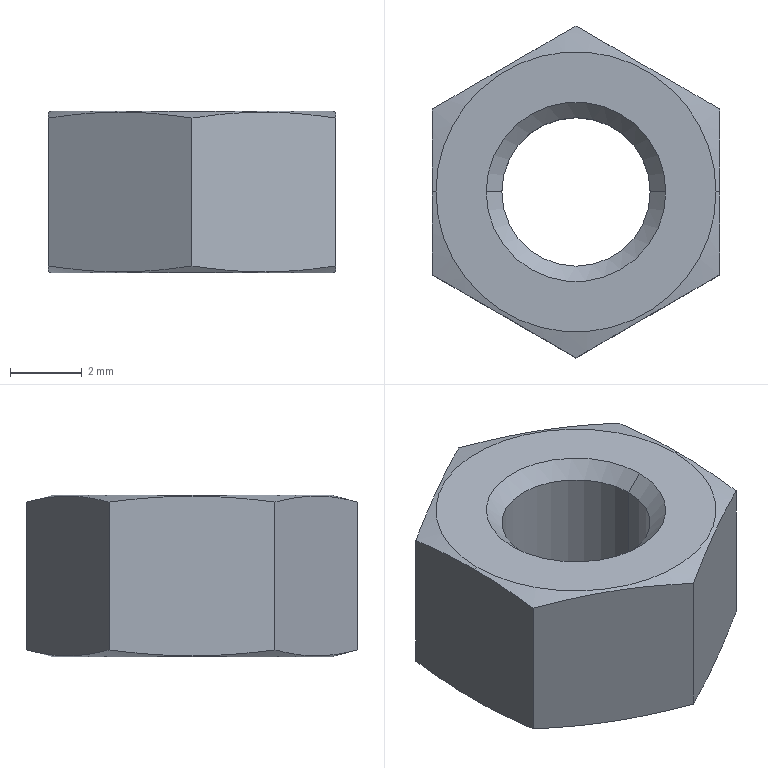Part | SolidWorks | features BaseBody 1 | 1 solid | 18 faces | box 8 x 9.238 x 4.5 mm | volume 185.536 mm3 | cone 8 | plane 8 | cylinder 2 | commonest cylinder face diameters 4.134 x2
STEP:
#1=CARTESIAN_POINT('',(-2.067,0.,-1.817));
#2=VERTEX_POINT('',#1);
#3=CARTESIAN_POINT('',(2.067,0.,-1.817));
#4=VERTEX_POINT('',#3);
#5=CARTESIAN_POINT('',(0.,0.,-1.817));
#6=DIRECTION('',(0.,0.,1.));
#7=DIRECTION('',(1.,0.,0.));
#8=AXIS2_PLACEMENT_3D('',#5,#6,#7);
#9=CIRCLE('',#8,2.067);
#10=EDGE_CURVE('',#2,#4,#9,.T.);
#11=ORIENTED_EDGE('',*,*,#10,.F.);
#12=CARTESIAN_POINT('',(-2.067,0.,1.817));
#13=VERTEX_POINT('',#12);
#14=CARTESIAN_POINT('',(-2.067,0.,-2.25));
#15=DIRECTION('',(0.,0.,1.));
#16=VECTOR('',#15,1000.);
#17=LINE('',#14,#16);
#18=EDGE_CURVE('',#2,#13,#17,.T.);
#19=ORIENTED_EDGE('',*,*,#18,.T.);
#20=CARTESIAN_POINT('',(2.067,0.,1.817));
#21=VERTEX_POINT('',#20);
#22=CARTESIAN_POINT('',(0.,0.,1.817));
#23=DIRECTION('',(0.,0.,-1.));
#24=DIRECTION('',(1.,0.,0.));
#25=AXIS2_PLACEMENT_3D('',#22,#23,#24);
#26=CIRCLE('',#25,2.067);
#27=EDGE_CURVE('',#21,#13,#26,.T.);
#28=ORIENTED_EDGE('',*,*,#27,.F.);
#29=CARTESIAN_POINT('',(2.067,0.,-2.25));
#30=DIRECTION('',(0.,0.,1.));
#31=VECTOR('',#30,1000.);
#32=LINE('',#29,#31);
#33=EDGE_CURVE('',#4,#21,#32,.T.);
#34=ORIENTED_EDGE('',*,*,#33,.F.);
#35=EDGE_LOOP('',(#11,#19,#28,#34));
#36=FACE_OUTER_BOUND('',#35,.T.);
#37=CARTESIAN_POINT('',(0.,0.,-2.25));
#38=DIRECTION('',(0.,0.,1.));
#39=DIRECTION('',(1.,0.,0.));
#40=AXIS2_PLACEMENT_3D('',#37,#38,#39);
#41=CYLINDRICAL_SURFACE('',#40,2.067);
#42=ADVANCED_FACE('',(#36),#41,.F.);
#43=ORIENTED_EDGE('',*,*,#27,.T.);
#44=CARTESIAN_POINT('',(-2.5,0.,2.25));
#45=VERTEX_POINT('',#44);
#46=CARTESIAN_POINT('',(-2.5,0.,2.25));
#47=DIRECTION('',(-0.7071,0.,0.7071));
#48=VECTOR('',#47,1000.);
#49=LINE('',#46,#48);
#50=EDGE_CURVE('',#13,#45,#49,.T.);
#51=ORIENTED_EDGE('',*,*,#50,.T.);
#52=CARTESIAN_POINT('',(2.5,0.,2.25));
#53=VERTEX_POINT('',#52);
#54=CARTESIAN_POINT('',(0.,0.,2.25));
#55=DIRECTION('',(0.,0.,-1.));
#56=DIRECTION('',(1.,0.,0.));
#57=AXIS2_PLACEMENT_3D('',#54,#55,#56);
#58=CIRCLE('',#57,2.5);
#59=EDGE_CURVE('',#53,#45,#58,.T.);
#60=ORIENTED_EDGE('',*,*,#59,.F.);
#61=CARTESIAN_POINT('',(2.5,0.,2.25));
#62=DIRECTION('',(0.7071,0.,0.7071));
#63=VECTOR('',#62,1000.);
#64=LINE('',#61,#63);
#65=EDGE_CURVE('',#21,#53,#64,.T.);
#66=ORIENTED_EDGE('',*,*,#65,.F.);
#67=EDGE_LOOP('',(#43,#51,#60,#66));
#68=FACE_OUTER_BOUND('',#67,.T.);
#69=CARTESIAN_POINT('',(0.,0.,2.25));
#70=DIRECTION('',(0.,0.,1.));
#71=DIRECTION('',(1.,0.,0.));
#72=AXIS2_PLACEMENT_3D('',#69,#70,#71);
#73=CONICAL_SURFACE('',#72,2.5,0.7854);
#74=ADVANCED_FACE('',(#68),#73,.F.);
#75=ORIENTED_EDGE('',*,*,#10,.T.);
#76=CARTESIAN_POINT('',(2.5,0.,-2.25));
#77=VERTEX_POINT('',#76);
#78=CARTESIAN_POINT('',(2.5,0.,-2.25));
#79=DIRECTION('',(0.7071,0.,-0.7071));
#80=VECTOR('',#79,1000.);
#81=LINE('',#78,#80);
#82=EDGE_CURVE('',#4,#77,#81,.T.);
#83=ORIENTED_EDGE('',*,*,#82,.T.);
#84=CARTESIAN_POINT('',(-2.5,0.,-2.25));
#85=VERTEX_POINT('',#84);
#86=CARTESIAN_POINT('',(0.,0.,-2.25));
#87=DIRECTION('',(0.,0.,1.));
#88=DIRECTION('',(-1.,0.,0.));
#89=AXIS2_PLACEMENT_3D('',#86,#87,#88);
#90=CIRCLE('',#89,2.5);
#91=EDGE_CURVE('',#85,#77,#90,.T.);
#92=ORIENTED_EDGE('',*,*,#91,.F.);
#93=CARTESIAN_POINT('',(-2.5,0.,-2.25));
#94=DIRECTION('',(-0.7071,0.,-0.7071));
#95=VECTOR('',#94,1000.);
#96=LINE('',#93,#95);
#97=EDGE_CURVE('',#2,#85,#96,.T.);
#98=ORIENTED_EDGE('',*,*,#97,.F.);
#99=EDGE_LOOP('',(#75,#83,#92,#98));
#100=FACE_OUTER_BOUND('',#99,.T.);
#101=CARTESIAN_POINT('',(0.,0.,-2.25));
#102=DIRECTION('',(0.,0.,-1.));
#103=DIRECTION('',(-1.,0.,0.));
#104=AXIS2_PLACEMENT_3D('',#101,#102,#103);
#105=CONICAL_SURFACE('',#104,2.5,0.7854);
#106=ADVANCED_FACE('',(#100),#105,.F.);
#107=CARTESIAN_POINT('',(-3.9,0.,2.25));
#108=VERTEX_POINT('',#107);
#109=CARTESIAN_POINT('',(3.9,0.,2.25));
#110=VERTEX_POINT('',#109);
#111=CARTESIAN_POINT('',(0.,0.,2.25));
#112=DIRECTION('',(0.,0.,-1.));
#113=DIRECTION('',(-1.,0.,0.));
#114=AXIS2_PLACEMENT_3D('',#111,#112,#113);
#115=CIRCLE('',#114,3.9);
#116=EDGE_CURVE('',#108,#110,#115,.T.);
#117=ORIENTED_EDGE('',*,*,#116,.T.);
#118=CARTESIAN_POINT('',(4.,0.,2.223));
#119=VERTEX_POINT('',#118);
#120=CARTESIAN_POINT('',(4.623,0.,2.056));
#121=DIRECTION('',(0.9659,0.,-0.2588));
#122=VECTOR('',#121,1000.);
#123=LINE('',#120,#122);
#124=EDGE_CURVE('',#110,#119,#123,.T.);
#125=ORIENTED_EDGE('',*,*,#124,.T.);
#126=CARTESIAN_POINT('',(4.,2.309,2.057));
#127=VERTEX_POINT('',#126);
#128=CARTESIAN_POINT('',(4.,0.,2.223));
#129=CARTESIAN_POINT('',(4.,0.7698,2.223));
#130=CARTESIAN_POINT('',(4.,1.54,2.161));
#131=CARTESIAN_POINT('',(4.,2.309,2.057));
#132=B_SPLINE_CURVE_WITH_KNOTS('',3,(#128,#129,#130,#131),.UNSPECIFIED.,.F.,.F.,(4,4),(0.002309,0.004619),.UNSPECIFIED.);
#133=EDGE_CURVE('',#119,#127,#132,.T.);
#134=ORIENTED_EDGE('',*,*,#133,.T.);
#135=CARTESIAN_POINT('',(0.000000042,4.619,2.057));
#136=VERTEX_POINT('',#135);
#137=CARTESIAN_POINT('',(4.,2.309,2.057));
#138=CARTESIAN_POINT('',(3.333,2.694,2.161));
#139=CARTESIAN_POINT('',(2.,3.464,2.286));
#140=CARTESIAN_POINT('',(0.6667,4.234,2.161));
#141=CARTESIAN_POINT('',(0.000000042,4.619,2.057));
#142=B_SPLINE_CURVE_WITH_KNOTS('',3,(#137,#138,#139,#140,#141),.UNSPECIFIED.,.F.,.F.,(4,1,4),(0.,0.002309,0.004619),.UNSPECIFIED.);
#143=EDGE_CURVE('',#127,#136,#142,.T.);
#144=ORIENTED_EDGE('',*,*,#143,.T.);
#145=CARTESIAN_POINT('',(-4.,2.309,2.057));
#146=VERTEX_POINT('',#145);
#147=CARTESIAN_POINT('',(0.000000042,4.619,2.057));
#148=CARTESIAN_POINT('',(-0.6667,4.234,2.161));
#149=CARTESIAN_POINT('',(-2.,3.464,2.286));
#150=CARTESIAN_POINT('',(-3.333,2.694,2.161));
#151=CARTESIAN_POINT('',(-4.,2.309,2.057));
#152=B_SPLINE_CURVE_WITH_KNOTS('',3,(#147,#148,#149,#150,#151),.UNSPECIFIED.,.F.,.F.,(4,1,4),(0.,0.002309,0.004619),.UNSPECIFIED.);
#153=EDGE_CURVE('',#136,#146,#152,.T.);
#154=ORIENTED_EDGE('',*,*,#153,.T.);
#155=CARTESIAN_POINT('',(-4.,0.,2.223));
#156=VERTEX_POINT('',#155);
#157=CARTESIAN_POINT('',(-4.,2.309,2.057));
#158=CARTESIAN_POINT('',(-4.,1.54,2.161));
#159=CARTESIAN_POINT('',(-4.,0.7698,2.223));
#160=CARTESIAN_POINT('',(-4.,0.,2.223));
#161=B_SPLINE_CURVE_WITH_KNOTS('',3,(#157,#158,#159,#160),.UNSPECIFIED.,.F.,.F.,(4,4),(0.,0.002309),.UNSPECIFIED.);
#162=EDGE_CURVE('',#146,#156,#161,.T.);
#163=ORIENTED_EDGE('',*,*,#162,.T.);
#164=CARTESIAN_POINT('',(-4.623,0.,2.056));
#165=DIRECTION('',(-0.9659,0.,-0.2588));
#166=VECTOR('',#165,1000.);
#167=LINE('',#164,#166);
#168=EDGE_CURVE('',#108,#156,#167,.T.);
#169=ORIENTED_EDGE('',*,*,#168,.F.);
#170=EDGE_LOOP('',(#117,#125,#134,#144,#154,#163,#169));
#171=FACE_OUTER_BOUND('',#170,.T.);
#172=CARTESIAN_POINT('',(0.,0.,2.056));
#173=DIRECTION('',(0.,0.,-1.));
#174=DIRECTION('',(-1.,0.,0.));
#175=AXIS2_PLACEMENT_3D('',#172,#173,#174);
#176=CONICAL_SURFACE('',#175,4.623,1.309);
#177=ADVANCED_FACE('',(#171),#176,.T.);
#178=CARTESIAN_POINT('',(3.9,0.,-2.25));
#179=VERTEX_POINT('',#178);
#180=CARTESIAN_POINT('',(-3.9,0.,-2.25));
#181=VERTEX_POINT('',#180);
#182=CARTESIAN_POINT('',(0.,0.,-2.25));
#183=DIRECTION('',(0.,0.,1.));
#184=DIRECTION('',(1.,0.,0.));
#185=AXIS2_PLACEMENT_3D('',#182,#183,#184);
#186=CIRCLE('',#185,3.9);
#187=EDGE_CURVE('',#179,#181,#186,.T.);
#188=ORIENTED_EDGE('',*,*,#187,.T.);
#189=CARTESIAN_POINT('',(-4.,0.,-2.223));
#190=VERTEX_POINT('',#189);
#191=CARTESIAN_POINT('',(-4.623,0.,-2.056));
#192=DIRECTION('',(-0.9659,0.,0.2588));
#193=VECTOR('',#192,1000.);
#194=LINE('',#191,#193);
#195=EDGE_CURVE('',#181,#190,#194,.T.);
#196=ORIENTED_EDGE('',*,*,#195,.T.);
#197=CARTESIAN_POINT('',(-4.,2.309,-2.057));
#198=VERTEX_POINT('',#197);
#199=CARTESIAN_POINT('',(-4.,0.,-2.223));
#200=CARTESIAN_POINT('',(-4.,0.7698,-2.223));
#201=CARTESIAN_POINT('',(-4.,1.54,-2.161));
#202=CARTESIAN_POINT('',(-4.,2.309,-2.057));
#203=B_SPLINE_CURVE_WITH_KNOTS('',3,(#199,#200,#201,#202),.UNSPECIFIED.,.F.,.F.,(4,4),(0.002309,0.004619),.UNSPECIFIED.);
#204=EDGE_CURVE('',#190,#198,#203,.T.);
#205=ORIENTED_EDGE('',*,*,#204,.T.);
#206=CARTESIAN_POINT('',(-0.000000042,4.619,-2.057));
#207=VERTEX_POINT('',#206);
#208=CARTESIAN_POINT('',(-4.,2.309,-2.057));
#209=CARTESIAN_POINT('',(-3.333,2.694,-2.161));
#210=CARTESIAN_POINT('',(-2.,3.464,-2.286));
#211=CARTESIAN_POINT('',(-0.6667,4.234,-2.161));
#212=CARTESIAN_POINT('',(-0.000000042,4.619,-2.057));
#213=B_SPLINE_CURVE_WITH_KNOTS('',3,(#208,#209,#210,#211,#212),.UNSPECIFIED.,.F.,.F.,(4,1,4),(0.,0.002309,0.004619),.UNSPECIFIED.);
#214=EDGE_CURVE('',#198,#207,#213,.T.);
#215=ORIENTED_EDGE('',*,*,#214,.T.);
#216=CARTESIAN_POINT('',(4.,2.309,-2.057));
#217=VERTEX_POINT('',#216);
#218=CARTESIAN_POINT('',(-0.000000042,4.619,-2.057));
#219=CARTESIAN_POINT('',(0.6667,4.234,-2.161));
#220=CARTESIAN_POINT('',(2.,3.464,-2.286));
#221=CARTESIAN_POINT('',(3.333,2.694,-2.161));
#222=CARTESIAN_POINT('',(4.,2.309,-2.057));
#223=B_SPLINE_CURVE_WITH_KNOTS('',3,(#218,#219,#220,#221,#222),.UNSPECIFIED.,.F.,.F.,(4,1,4),(0.,0.002309,0.004619),.UNSPECIFIED.);
#224=EDGE_CURVE('',#207,#217,#223,.T.);
#225=ORIENTED_EDGE('',*,*,#224,.T.);
#226=CARTESIAN_POINT('',(4.,0.,-2.223));
#227=VERTEX_POINT('',#226);
#228=CARTESIAN_POINT('',(4.,2.309,-2.057));
#229=CARTESIAN_POINT('',(4.,1.54,-2.161));
#230=CARTESIAN_POINT('',(4.,0.7698,-2.223));
#231=CARTESIAN_POINT('',(4.,0.,-2.223));
#232=B_SPLINE_CURVE_WITH_KNOTS('',3,(#228,#229,#230,#231),.UNSPECIFIED.,.F.,.F.,(4,4),(0.,0.002309),.UNSPECIFIED.);
#233=EDGE_CURVE('',#217,#227,#232,.T.);
#234=ORIENTED_EDGE('',*,*,#233,.T.);
#235=CARTESIAN_POINT('',(4.623,0.,-2.056));
#236=DIRECTION('',(0.9659,0.,0.2588));
#237=VECTOR('',#236,1000.);
#238=LINE('',#235,#237);
#239=EDGE_CURVE('',#179,#227,#238,.T.);
#240=ORIENTED_EDGE('',*,*,#239,.F.);
#241=EDGE_LOOP('',(#188,#196,#205,#215,#225,#234,#240));
#242=FACE_OUTER_BOUND('',#241,.T.);
#243=CARTESIAN_POINT('',(0.,0.,-2.056));
#244=DIRECTION('',(0.,0.,1.));
#245=DIRECTION('',(1.,0.,0.));
#246=AXIS2_PLACEMENT_3D('',#243,#244,#245);
#247=CONICAL_SURFACE('',#246,4.623,1.309);
#248=ADVANCED_FACE('',(#242),#247,.T.);
#249=ORIENTED_EDGE('',*,*,#18,.F.);
#250=CARTESIAN_POINT('',(0.,0.,-1.817));
#251=DIRECTION('',(0.,0.,1.));
#252=DIRECTION('',(1.,0.,0.));
#253=AXIS2_PLACEMENT_3D('',#250,#251,#252);
#254=CIRCLE('',#253,2.067);
#255=EDGE_CURVE('',#4,#2,#254,.T.);
#256=ORIENTED_EDGE('',*,*,#255,.F.);
#257=ORIENTED_EDGE('',*,*,#33,.T.);
#258=CARTESIAN_POINT('',(0.,0.,1.817));
#259=DIRECTION('',(0.,0.,-1.));
#260=DIRECTION('',(1.,0.,0.));
#261=AXIS2_PLACEMENT_3D('',#258,#259,#260);
#262=CIRCLE('',#261,2.067);
#263=EDGE_CURVE('',#13,#21,#262,.T.);
#264=ORIENTED_EDGE('',*,*,#263,.F.);
#265=EDGE_LOOP('',(#249,#256,#257,#264));
#266=FACE_OUTER_BOUND('',#265,.T.);
#267=CARTESIAN_POINT('',(0.,0.,-2.25));
#268=DIRECTION('',(0.,0.,1.));
#269=DIRECTION('',(1.,0.,0.));
#270=AXIS2_PLACEMENT_3D('',#267,#268,#269);
#271=CYLINDRICAL_SURFACE('',#270,2.067);
#272=ADVANCED_FACE('',(#266),#271,.F.);
#273=ORIENTED_EDGE('',*,*,#50,.F.);
#274=ORIENTED_EDGE('',*,*,#263,.T.);
#275=ORIENTED_EDGE('',*,*,#65,.T.);
#276=CARTESIAN_POINT('',(0.,0.,2.25));
#277=DIRECTION('',(0.,0.,-1.));
#278=DIRECTION('',(1.,0.,0.));
#279=AXIS2_PLACEMENT_3D('',#276,#277,#278);
#280=CIRCLE('',#279,2.5);
#281=EDGE_CURVE('',#45,#53,#280,.T.);
#282=ORIENTED_EDGE('',*,*,#281,.F.);
#283=EDGE_LOOP('',(#273,#274,#275,#282));
#284=FACE_OUTER_BOUND('',#283,.T.);
#285=CARTESIAN_POINT('',(0.,0.,2.25));
#286=DIRECTION('',(0.,0.,1.));
#287=DIRECTION('',(1.,0.,0.));
#288=AXIS2_PLACEMENT_3D('',#285,#286,#287);
#289=CONICAL_SURFACE('',#288,2.5,0.7854);
#290=ADVANCED_FACE('',(#284),#289,.F.);
#291=ORIENTED_EDGE('',*,*,#82,.F.);
#292=ORIENTED_EDGE('',*,*,#255,.T.);
#293=ORIENTED_EDGE('',*,*,#97,.T.);
#294=CARTESIAN_POINT('',(0.,0.,-2.25));
#295=DIRECTION('',(0.,0.,1.));
#296=DIRECTION('',(-1.,0.,0.));
#297=AXIS2_PLACEMENT_3D('',#294,#295,#296);
#298=CIRCLE('',#297,2.5);
#299=EDGE_CURVE('',#77,#85,#298,.T.);
#300=ORIENTED_EDGE('',*,*,#299,.F.);
#301=EDGE_LOOP('',(#291,#292,#293,#300));
#302=FACE_OUTER_BOUND('',#301,.T.);
#303=CARTESIAN_POINT('',(0.,0.,-2.25));
#304=DIRECTION('',(0.,0.,-1.));
#305=DIRECTION('',(-1.,0.,0.));
#306=AXIS2_PLACEMENT_3D('',#303,#304,#305);
#307=CONICAL_SURFACE('',#306,2.5,0.7854);
#308=ADVANCED_FACE('',(#302),#307,.F.);
#309=ORIENTED_EDGE('',*,*,#59,.T.);
#310=ORIENTED_EDGE('',*,*,#281,.T.);
#311=EDGE_LOOP('',(#309,#310));
#312=FACE_BOUND('',#311,.T.);
#313=ORIENTED_EDGE('',*,*,#116,.F.);
#314=CARTESIAN_POINT('',(0.,0.,2.25));
#315=DIRECTION('',(0.,0.,-1.));
#316=DIRECTION('',(-1.,0.,0.));
#317=AXIS2_PLACEMENT_3D('',#314,#315,#316);
#318=CIRCLE('',#317,3.9);
#319=EDGE_CURVE('',#110,#108,#318,.T.);
#320=ORIENTED_EDGE('',*,*,#319,.F.);
#321=EDGE_LOOP('',(#313,#320));
#322=FACE_OUTER_BOUND('',#321,.T.);
#323=CARTESIAN_POINT('',(0.,0.,2.25));
#324=DIRECTION('',(0.,0.,-1.));
#325=DIRECTION('',(-1.,0.,0.));
#326=AXIS2_PLACEMENT_3D('',#323,#324,#325);
#327=PLANE('',#326);
#328=ADVANCED_FACE('',(#312,#322),#327,.F.);
#329=ORIENTED_EDGE('',*,*,#187,.F.);
#330=CARTESIAN_POINT('',(0.,0.,-2.25));
#331=DIRECTION('',(0.,0.,1.));
#332=DIRECTION('',(1.,0.,0.));
#333=AXIS2_PLACEMENT_3D('',#330,#331,#332);
#334=CIRCLE('',#333,3.9);
#335=EDGE_CURVE('',#181,#179,#334,.T.);
#336=ORIENTED_EDGE('',*,*,#335,.F.);
#337=EDGE_LOOP('',(#329,#336));
#338=FACE_OUTER_BOUND('',#337,.T.);
#339=ORIENTED_EDGE('',*,*,#91,.T.);
#340=ORIENTED_EDGE('',*,*,#299,.T.);
#341=EDGE_LOOP('',(#339,#340));
#342=FACE_BOUND('',#341,.T.);
#343=CARTESIAN_POINT('',(0.,3.9,-2.25));
#344=DIRECTION('',(0.,0.,1.));
#345=DIRECTION('',(1.,0.,0.));
#346=AXIS2_PLACEMENT_3D('',#343,#344,#345);
#347=PLANE('',#346);
#348=ADVANCED_FACE('',(#338,#342),#347,.F.);
#349=ORIENTED_EDGE('',*,*,#124,.F.);
#350=ORIENTED_EDGE('',*,*,#319,.T.);
#351=ORIENTED_EDGE('',*,*,#168,.T.);
#352=CARTESIAN_POINT('',(-4.,-2.309,2.057));
#353=VERTEX_POINT('',#352);
#354=CARTESIAN_POINT('',(-4.,0.,2.223));
#355=CARTESIAN_POINT('',(-4.,-0.7698,2.223));
#356=CARTESIAN_POINT('',(-4.,-1.54,2.161));
#357=CARTESIAN_POINT('',(-4.,-2.309,2.057));
#358=B_SPLINE_CURVE_WITH_KNOTS('',3,(#354,#355,#356,#357),.UNSPECIFIED.,.F.,.F.,(4,4),(0.002309,0.004619),.UNSPECIFIED.);
#359=EDGE_CURVE('',#156,#353,#358,.T.);
#360=ORIENTED_EDGE('',*,*,#359,.T.);
#361=CARTESIAN_POINT('',(-0.000000042,-4.619,2.057));
#362=VERTEX_POINT('',#361);
#363=CARTESIAN_POINT('',(-4.,-2.309,2.057));
#364=CARTESIAN_POINT('',(-3.333,-2.694,2.161));
#365=CARTESIAN_POINT('',(-2.,-3.464,2.286));
#366=CARTESIAN_POINT('',(-0.6667,-4.234,2.161));
#367=CARTESIAN_POINT('',(-0.000000042,-4.619,2.057));
#368=B_SPLINE_CURVE_WITH_KNOTS('',3,(#363,#364,#365,#366,#367),.UNSPECIFIED.,.F.,.F.,(4,1,4),(0.,0.002309,0.004619),.UNSPECIFIED.);
#369=EDGE_CURVE('',#353,#362,#368,.T.);
#370=ORIENTED_EDGE('',*,*,#369,.T.);
#371=CARTESIAN_POINT('',(4.,-2.309,2.057));
#372=VERTEX_POINT('',#371);
#373=CARTESIAN_POINT('',(-0.000000042,-4.619,2.057));
#374=CARTESIAN_POINT('',(0.6667,-4.234,2.161));
#375=CARTESIAN_POINT('',(2.,-3.464,2.286));
#376=CARTESIAN_POINT('',(3.333,-2.694,2.161));
#377=CARTESIAN_POINT('',(4.,-2.309,2.057));
#378=B_SPLINE_CURVE_WITH_KNOTS('',3,(#373,#374,#375,#376,#377),.UNSPECIFIED.,.F.,.F.,(4,1,4),(0.,0.002309,0.004619),.UNSPECIFIED.);
#379=EDGE_CURVE('',#362,#372,#378,.T.);
#380=ORIENTED_EDGE('',*,*,#379,.T.);
#381=CARTESIAN_POINT('',(4.,-2.309,2.057));
#382=CARTESIAN_POINT('',(4.,-1.54,2.161));
#383=CARTESIAN_POINT('',(4.,-0.7698,2.223));
#384=CARTESIAN_POINT('',(4.,0.,2.223));
#385=B_SPLINE_CURVE_WITH_KNOTS('',3,(#381,#382,#383,#384),.UNSPECIFIED.,.F.,.F.,(4,4),(0.,0.002309),.UNSPECIFIED.);
#386=EDGE_CURVE('',#372,#119,#385,.T.);
#387=ORIENTED_EDGE('',*,*,#386,.T.);
#388=EDGE_LOOP('',(#349,#350,#351,#360,#370,#380,#387));
#389=FACE_OUTER_BOUND('',#388,.T.);
#390=CARTESIAN_POINT('',(0.,0.,2.056));
#391=DIRECTION('',(0.,0.,-1.));
#392=DIRECTION('',(-1.,0.,0.));
#393=AXIS2_PLACEMENT_3D('',#390,#391,#392);
#394=CONICAL_SURFACE('',#393,4.623,1.309);
#395=ADVANCED_FACE('',(#389),#394,.T.);
#396=ORIENTED_EDGE('',*,*,#195,.F.);
#397=ORIENTED_EDGE('',*,*,#335,.T.);
#398=ORIENTED_EDGE('',*,*,#239,.T.);
#399=CARTESIAN_POINT('',(4.,-2.309,-2.057));
#400=VERTEX_POINT('',#399);
#401=CARTESIAN_POINT('',(4.,0.,-2.223));
#402=CARTESIAN_POINT('',(4.,-0.7698,-2.223));
#403=CARTESIAN_POINT('',(4.,-1.54,-2.161));
#404=CARTESIAN_POINT('',(4.,-2.309,-2.057));
#405=B_SPLINE_CURVE_WITH_KNOTS('',3,(#401,#402,#403,#404),.UNSPECIFIED.,.F.,.F.,(4,4),(0.002309,0.004619),.UNSPECIFIED.);
#406=EDGE_CURVE('',#227,#400,#405,.T.);
#407=ORIENTED_EDGE('',*,*,#406,.T.);
#408=CARTESIAN_POINT('',(-0.00000002,-4.619,-2.057));
#409=VERTEX_POINT('',#408);
#410=CARTESIAN_POINT('',(4.,-2.309,-2.057));
#411=CARTESIAN_POINT('',(3.333,-2.694,-2.161));
#412=CARTESIAN_POINT('',(2.,-3.464,-2.286));
#413=CARTESIAN_POINT('',(0.6667,-4.234,-2.161));
#414=CARTESIAN_POINT('',(-0.00000002,-4.619,-2.057));
#415=B_SPLINE_CURVE_WITH_KNOTS('',3,(#410,#411,#412,#413,#414),.UNSPECIFIED.,.F.,.F.,(4,1,4),(0.,0.002309,0.004619),.UNSPECIFIED.);
#416=EDGE_CURVE('',#400,#409,#415,.T.);
#417=ORIENTED_EDGE('',*,*,#416,.T.);
#418=CARTESIAN_POINT('',(-4.,-2.309,-2.057));
#419=VERTEX_POINT('',#418);
#420=CARTESIAN_POINT('',(-0.00000002,-4.619,-2.057));
#421=CARTESIAN_POINT('',(-0.6667,-4.234,-2.161));
#422=CARTESIAN_POINT('',(-2.,-3.464,-2.286));
#423=CARTESIAN_POINT('',(-3.333,-2.694,-2.161));
#424=CARTESIAN_POINT('',(-4.,-2.309,-2.057));
#425=B_SPLINE_CURVE_WITH_KNOTS('',3,(#420,#421,#422,#423,#424),.UNSPECIFIED.,.F.,.F.,(4,1,4),(0.,0.002309,0.004619),.UNSPECIFIED.);
#426=EDGE_CURVE('',#409,#419,#425,.T.);
#427=ORIENTED_EDGE('',*,*,#426,.T.);
#428=CARTESIAN_POINT('',(-4.,-2.309,-2.057));
#429=CARTESIAN_POINT('',(-4.,-1.54,-2.161));
#430=CARTESIAN_POINT('',(-4.,-0.7698,-2.223));
#431=CARTESIAN_POINT('',(-4.,0.,-2.223));
#432=B_SPLINE_CURVE_WITH_KNOTS('',3,(#428,#429,#430,#431),.UNSPECIFIED.,.F.,.F.,(4,4),(0.,0.002309),.UNSPECIFIED.);
#433=EDGE_CURVE('',#419,#190,#432,.T.);
#434=ORIENTED_EDGE('',*,*,#433,.T.);
#435=EDGE_LOOP('',(#396,#397,#398,#407,#417,#427,#434));
#436=FACE_OUTER_BOUND('',#435,.T.);
#437=CARTESIAN_POINT('',(0.,0.,-2.056));
#438=DIRECTION('',(0.,0.,1.));
#439=DIRECTION('',(1.,0.,0.));
#440=AXIS2_PLACEMENT_3D('',#437,#438,#439);
#441=CONICAL_SURFACE('',#440,4.623,1.309);
#442=ADVANCED_FACE('',(#436),#441,.T.);
#443=ORIENTED_EDGE('',*,*,#233,.F.);
#444=CARTESIAN_POINT('',(4.,2.309,2.25));
#445=DIRECTION('',(0.,0.,-1.));
#446=VECTOR('',#445,1000.);
#447=LINE('',#444,#446);
#448=EDGE_CURVE('',#127,#217,#447,.T.);
#449=ORIENTED_EDGE('',*,*,#448,.F.);
#450=ORIENTED_EDGE('',*,*,#133,.F.);
#451=ORIENTED_EDGE('',*,*,#386,.F.);
#452=CARTESIAN_POINT('',(4.,-2.309,2.25));
#453=DIRECTION('',(0.,0.,1.));
#454=VECTOR('',#453,1000.);
#455=LINE('',#452,#454);
#456=EDGE_CURVE('',#400,#372,#455,.T.);
#457=ORIENTED_EDGE('',*,*,#456,.F.);
#458=ORIENTED_EDGE('',*,*,#406,.F.);
#459=EDGE_LOOP('',(#443,#449,#450,#451,#457,#458));
#460=FACE_OUTER_BOUND('',#459,.T.);
#461=CARTESIAN_POINT('',(4.,-2.309,2.25));
#462=DIRECTION('',(-1.,0.,0.));
#463=DIRECTION('',(0.,0.,1.));
#464=AXIS2_PLACEMENT_3D('',#461,#462,#463);
#465=PLANE('',#464);
#466=ADVANCED_FACE('',(#460),#465,.F.);
#467=ORIENTED_EDGE('',*,*,#416,.F.);
#468=ORIENTED_EDGE('',*,*,#456,.T.);
#469=ORIENTED_EDGE('',*,*,#379,.F.);
#470=CARTESIAN_POINT('',(0.,-4.619,2.25));
#471=DIRECTION('',(0.,0.,1.));
#472=VECTOR('',#471,1000.);
#473=LINE('',#470,#472);
#474=EDGE_CURVE('',#409,#362,#473,.T.);
#475=ORIENTED_EDGE('',*,*,#474,.F.);
#476=EDGE_LOOP('',(#467,#468,#469,#475));
#477=FACE_OUTER_BOUND('',#476,.T.);
#478=CARTESIAN_POINT('',(0.,-4.619,2.25));
#479=DIRECTION('',(-0.5,0.866,0.));
#480=DIRECTION('',(-0.866,-0.5,0.));
#481=AXIS2_PLACEMENT_3D('',#478,#479,#480);
#482=PLANE('',#481);
#483=ADVANCED_FACE('',(#477),#482,.F.);
#484=ORIENTED_EDGE('',*,*,#426,.F.);
#485=ORIENTED_EDGE('',*,*,#474,.T.);
#486=ORIENTED_EDGE('',*,*,#369,.F.);
#487=CARTESIAN_POINT('',(-4.,-2.309,2.25));
#488=DIRECTION('',(0.,0.,1.));
#489=VECTOR('',#488,1000.);
#490=LINE('',#487,#489);
#491=EDGE_CURVE('',#419,#353,#490,.T.);
#492=ORIENTED_EDGE('',*,*,#491,.F.);
#493=EDGE_LOOP('',(#484,#485,#486,#492));
#494=FACE_OUTER_BOUND('',#493,.T.);
#495=CARTESIAN_POINT('',(-4.,-2.309,2.25));
#496=DIRECTION('',(0.5,0.866,0.));
#497=DIRECTION('',(-0.866,0.5,0.));
#498=AXIS2_PLACEMENT_3D('',#495,#496,#497);
#499=PLANE('',#498);
#500=ADVANCED_FACE('',(#494),#499,.F.);
#501=ORIENTED_EDGE('',*,*,#433,.F.);
#502=ORIENTED_EDGE('',*,*,#491,.T.);
#503=ORIENTED_EDGE('',*,*,#359,.F.);
#504=ORIENTED_EDGE('',*,*,#162,.F.);
#505=CARTESIAN_POINT('',(-4.,2.309,2.25));
#506=DIRECTION('',(0.,0.,1.));
#507=VECTOR('',#506,1000.);
#508=LINE('',#505,#507);
#509=EDGE_CURVE('',#198,#146,#508,.T.);
#510=ORIENTED_EDGE('',*,*,#509,.F.);
#511=ORIENTED_EDGE('',*,*,#204,.F.);
#512=EDGE_LOOP('',(#501,#502,#503,#504,#510,#511));
#513=FACE_OUTER_BOUND('',#512,.T.);
#514=CARTESIAN_POINT('',(-4.,2.309,2.25));
#515=DIRECTION('',(1.,0.,0.));
#516=DIRECTION('',(0.,0.,-1.));
#517=AXIS2_PLACEMENT_3D('',#514,#515,#516);
#518=PLANE('',#517);
#519=ADVANCED_FACE('',(#513),#518,.F.);
#520=ORIENTED_EDGE('',*,*,#214,.F.);
#521=ORIENTED_EDGE('',*,*,#509,.T.);
#522=ORIENTED_EDGE('',*,*,#153,.F.);
#523=CARTESIAN_POINT('',(0.,4.619,2.25));
#524=DIRECTION('',(0.,0.,1.));
#525=VECTOR('',#524,1000.);
#526=LINE('',#523,#525);
#527=EDGE_CURVE('',#207,#136,#526,.T.);
#528=ORIENTED_EDGE('',*,*,#527,.F.);
#529=EDGE_LOOP('',(#520,#521,#522,#528));
#530=FACE_OUTER_BOUND('',#529,.T.);
#531=CARTESIAN_POINT('',(0.,4.619,2.25));
#532=DIRECTION('',(0.5,-0.866,0.));
#533=DIRECTION('',(0.866,0.5,0.));
#534=AXIS2_PLACEMENT_3D('',#531,#532,#533);
#535=PLANE('',#534);
#536=ADVANCED_FACE('',(#530),#535,.F.);
#537=ORIENTED_EDGE('',*,*,#224,.F.);
#538=ORIENTED_EDGE('',*,*,#527,.T.);
#539=ORIENTED_EDGE('',*,*,#143,.F.);
#540=ORIENTED_EDGE('',*,*,#448,.T.);
#541=EDGE_LOOP('',(#537,#538,#539,#540));
#542=FACE_OUTER_BOUND('',#541,.T.);
#543=CARTESIAN_POINT('',(4.,2.309,2.25));
#544=DIRECTION('',(-0.5,-0.866,0.));
#545=DIRECTION('',(0.866,-0.5,0.));
#546=AXIS2_PLACEMENT_3D('',#543,#544,#545);
#547=PLANE('',#546);
#548=ADVANCED_FACE('',(#542),#547,.F.);
#549=CLOSED_SHELL('',(#42,#74,#106,#177,#248,#272,#290,#308,#328,#348,#395,#442,#466,#483,#500,#519,#536,#548));
#550=MANIFOLD_SOLID_BREP('',#549);
#551=CARTESIAN_POINT('',(0.,0.,0.));
#552=DIRECTION('',(0.,0.,1.));
#553=DIRECTION('',(1.,0.,0.));
#554=AXIS2_PLACEMENT_3D('',#551,#552,#553);
#555=(LENGTH_UNIT()NAMED_UNIT(*)SI_UNIT(.MILLI.,.METRE.));
#556=UNCERTAINTY_MEASURE_WITH_UNIT(LENGTH_MEASURE(0.00001),#555,'','');
#557=(NAMED_UNIT(*)PLANE_ANGLE_UNIT()SI_UNIT($,.RADIAN.));
#558=(NAMED_UNIT(*)SI_UNIT($,.STERADIAN.)SOLID_ANGLE_UNIT());
#559=(GEOMETRIC_REPRESENTATION_CONTEXT(3)GLOBAL_UNCERTAINTY_ASSIGNED_CONTEXT((#556))GLOBAL_UNIT_ASSIGNED_CONTEXT((#555,#557,#558))REPRESENTATION_CONTEXT('',''));
#560=ADVANCED_BREP_SHAPE_REPRESENTATION('',(#550,#554),#559);